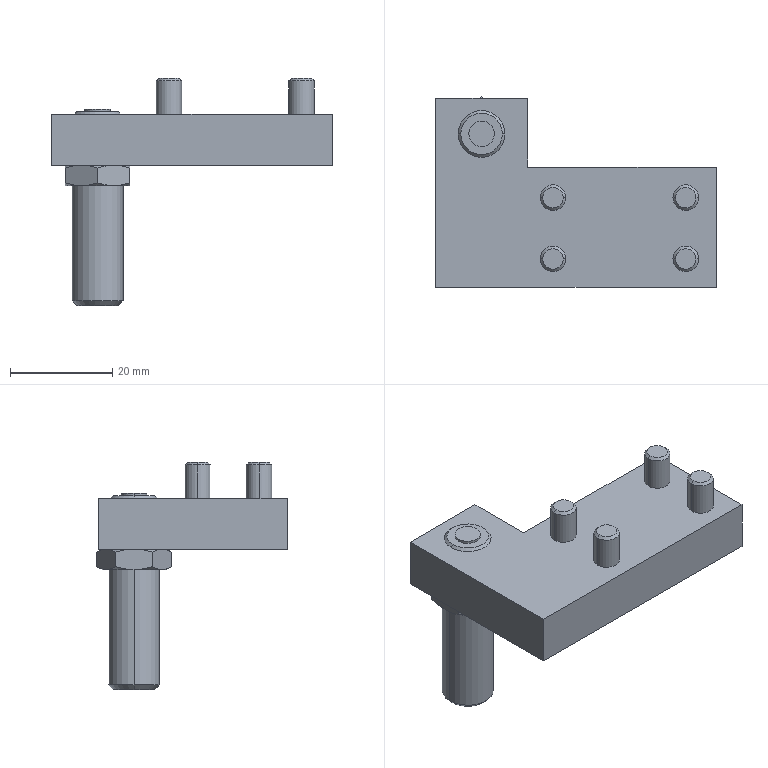Part | SolidWorks | features BaseBody 1 | 1 solid | 98 faces | box 55 x 37.275 x 44.5 mm | volume 18284 mm3 | plane 54 | cylinder 20 | cone 16 | spline 8 | commonest cylinder face diameters 5 x10 9 x8 10 x2